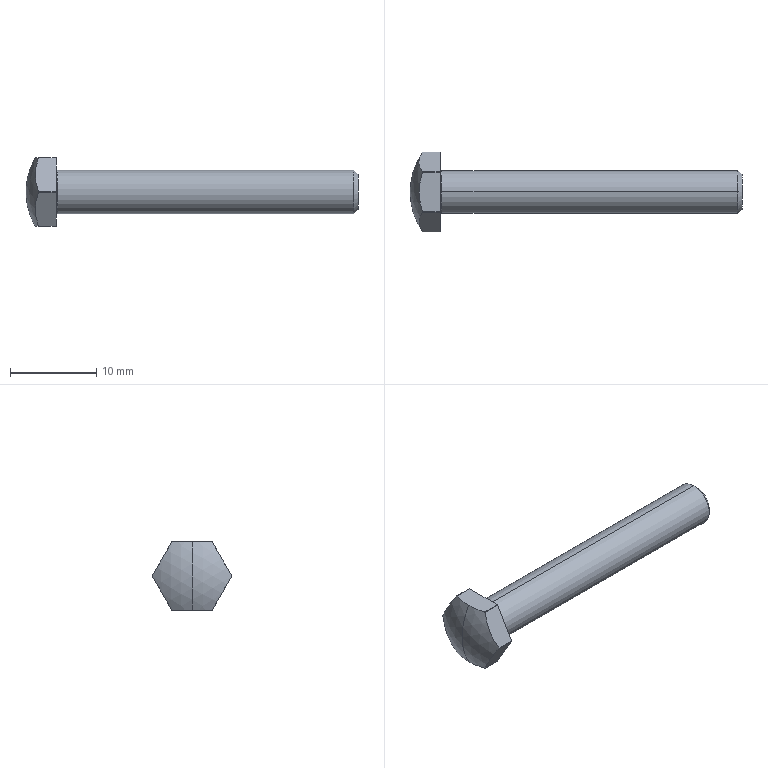Part | STEP file | 11-F12906-LQ-STBB5_35bA11 | 1 solid | 22 faces | box 38.5 x 9.2 x 8 mm | volume 847.17 mm3 | cylinder 8 | plane 8 | cone 2 | torus 2 | sphere 2 | commonest cylinder face diameters 9.2 x6 5 x2
STEP:
#1=CARTESIAN_POINT('',(35.,0.,2.01));
#2=VERTEX_POINT('',#1);
#3=CARTESIAN_POINT('',(35.,0.,-2.01));
#4=VERTEX_POINT('',#3);
#5=CARTESIAN_POINT('',(35.,0.,0.));
#6=DIRECTION('',(-1.,0.,0.));
#7=DIRECTION('',(0.,0.,1.));
#8=AXIS2_PLACEMENT_3D('',#5,#6,#7);
#9=CIRCLE('',#8,2.01);
#10=EDGE_CURVE('',#2,#4,#9,.T.);
#11=ORIENTED_EDGE('',*,*,#10,.T.);
#12=CARTESIAN_POINT('',(34.51,0.,-2.5));
#13=VERTEX_POINT('',#12);
#14=CARTESIAN_POINT('',(35.,0.,-2.01));
#15=DIRECTION('',(-0.7071,0.,-0.7071));
#16=VECTOR('',#15,1000.);
#17=LINE('',#14,#16);
#18=EDGE_CURVE('',#4,#13,#17,.T.);
#19=ORIENTED_EDGE('',*,*,#18,.T.);
#20=CARTESIAN_POINT('',(34.51,0.,2.5));
#21=VERTEX_POINT('',#20);
#22=CARTESIAN_POINT('',(34.51,0.,0.));
#23=DIRECTION('',(-1.,0.,0.));
#24=DIRECTION('',(0.,0.,1.));
#25=AXIS2_PLACEMENT_3D('',#22,#23,#24);
#26=CIRCLE('',#25,2.5);
#27=EDGE_CURVE('',#21,#13,#26,.T.);
#28=ORIENTED_EDGE('',*,*,#27,.F.);
#29=CARTESIAN_POINT('',(35.,0.,2.01));
#30=DIRECTION('',(-0.7071,0.,0.7071));
#31=VECTOR('',#30,1000.);
#32=LINE('',#29,#31);
#33=EDGE_CURVE('',#2,#21,#32,.T.);
#34=ORIENTED_EDGE('',*,*,#33,.F.);
#35=EDGE_LOOP('',(#11,#19,#28,#34));
#36=FACE_OUTER_BOUND('',#35,.T.);
#37=CARTESIAN_POINT('',(35.,0.,0.));
#38=DIRECTION('',(-1.,0.,0.));
#39=DIRECTION('',(0.,0.,1.));
#40=AXIS2_PLACEMENT_3D('',#37,#38,#39);
#41=CONICAL_SURFACE('',#40,2.01,0.7854);
#42=ADVANCED_FACE('',(#36),#41,.T.);
#43=ORIENTED_EDGE('',*,*,#27,.T.);
#44=CARTESIAN_POINT('',(0.2,0.,-2.5));
#45=VERTEX_POINT('',#44);
#46=CARTESIAN_POINT('',(35.,0.,-2.5));
#47=DIRECTION('',(-1.,0.,0.));
#48=VECTOR('',#47,1000.);
#49=LINE('',#46,#48);
#50=EDGE_CURVE('',#13,#45,#49,.T.);
#51=ORIENTED_EDGE('',*,*,#50,.T.);
#52=CARTESIAN_POINT('',(0.2,0.,2.5));
#53=VERTEX_POINT('',#52);
#54=CARTESIAN_POINT('',(0.2,0.,0.));
#55=DIRECTION('',(-1.,0.,0.));
#56=DIRECTION('',(0.,0.,1.));
#57=AXIS2_PLACEMENT_3D('',#54,#55,#56);
#58=CIRCLE('',#57,2.5);
#59=EDGE_CURVE('',#53,#45,#58,.T.);
#60=ORIENTED_EDGE('',*,*,#59,.F.);
#61=CARTESIAN_POINT('',(35.,0.,2.5));
#62=DIRECTION('',(-1.,0.,0.));
#63=VECTOR('',#62,1000.);
#64=LINE('',#61,#63);
#65=EDGE_CURVE('',#21,#53,#64,.T.);
#66=ORIENTED_EDGE('',*,*,#65,.F.);
#67=EDGE_LOOP('',(#43,#51,#60,#66));
#68=FACE_OUTER_BOUND('',#67,.T.);
#69=CARTESIAN_POINT('',(35.,0.,0.));
#70=DIRECTION('',(-1.,0.,0.));
#71=DIRECTION('',(0.,0.,1.));
#72=AXIS2_PLACEMENT_3D('',#69,#70,#71);
#73=CYLINDRICAL_SURFACE('',#72,2.5);
#74=ADVANCED_FACE('',(#68),#73,.T.);
#75=CARTESIAN_POINT('',(0.,0.,-2.7));
#76=VERTEX_POINT('',#75);
#77=CARTESIAN_POINT('',(0.,0.,2.7));
#78=VERTEX_POINT('',#77);
#79=CARTESIAN_POINT('',(0.,0.,0.));
#80=DIRECTION('',(-1.,0.,0.));
#81=DIRECTION('',(0.,0.,1.));
#82=AXIS2_PLACEMENT_3D('',#79,#80,#81);
#83=CIRCLE('',#82,2.7);
#84=EDGE_CURVE('',#76,#78,#83,.T.);
#85=ORIENTED_EDGE('',*,*,#84,.F.);
#86=CARTESIAN_POINT('',(0.2,0.,-2.7));
#87=DIRECTION('',(0.,1.,0.));
#88=DIRECTION('',(0.,0.,1.));
#89=AXIS2_PLACEMENT_3D('',#86,#87,#88);
#90=CIRCLE('',#89,0.2);
#91=EDGE_CURVE('',#76,#45,#90,.T.);
#92=ORIENTED_EDGE('',*,*,#91,.T.);
#93=CARTESIAN_POINT('',(0.2,0.,0.));
#94=DIRECTION('',(-1.,0.,0.));
#95=DIRECTION('',(0.,0.,1.));
#96=AXIS2_PLACEMENT_3D('',#93,#94,#95);
#97=CIRCLE('',#96,2.5);
#98=EDGE_CURVE('',#45,#53,#97,.T.);
#99=ORIENTED_EDGE('',*,*,#98,.T.);
#100=CARTESIAN_POINT('',(0.2,0.,2.7));
#101=DIRECTION('',(0.,-1.,0.));
#102=DIRECTION('',(0.,0.,-1.));
#103=AXIS2_PLACEMENT_3D('',#100,#101,#102);
#104=CIRCLE('',#103,0.2);
#105=EDGE_CURVE('',#78,#53,#104,.T.);
#106=ORIENTED_EDGE('',*,*,#105,.F.);
#107=EDGE_LOOP('',(#85,#92,#99,#106));
#108=FACE_OUTER_BOUND('',#107,.T.);
#109=CARTESIAN_POINT('',(0.2,0.,0.));
#110=DIRECTION('',(-1.,0.,0.));
#111=DIRECTION('',(0.,0.,1.));
#112=AXIS2_PLACEMENT_3D('',#109,#110,#111);
#113=TOROIDAL_SURFACE('',#112,2.7,0.2);
#114=ADVANCED_FACE('',(#108),#113,.F.);
#115=CARTESIAN_POINT('',(-2.428,0.,4.));
#116=VERTEX_POINT('',#115);
#117=CARTESIAN_POINT('',(-2.045,-2.272,4.));
#118=VERTEX_POINT('',#117);
#119=CARTESIAN_POINT('',(4.5,0.,4.));
#120=DIRECTION('',(0.,0.,1.));
#121=DIRECTION('',(1.,0.,0.));
#122=AXIS2_PLACEMENT_3D('',#119,#120,#121);
#123=CIRCLE('',#122,6.928);
#124=EDGE_CURVE('',#116,#118,#123,.T.);
#125=ORIENTED_EDGE('',*,*,#124,.F.);
#126=CARTESIAN_POINT('',(-3.5,0.,0.));
#127=VERTEX_POINT('',#126);
#128=CARTESIAN_POINT('',(4.5,0.,0.));
#129=DIRECTION('',(0.,-1.,0.));
#130=DIRECTION('',(0.,0.,-1.));
#131=AXIS2_PLACEMENT_3D('',#128,#129,#130);
#132=CIRCLE('',#131,8.);
#133=EDGE_CURVE('',#116,#127,#132,.T.);
#134=ORIENTED_EDGE('',*,*,#133,.T.);
#135=CARTESIAN_POINT('',(-2.428,0.,-4.));
#136=VERTEX_POINT('',#135);
#137=CARTESIAN_POINT('',(4.5,0.,0.));
#138=DIRECTION('',(0.,1.,0.));
#139=DIRECTION('',(0.,0.,1.));
#140=AXIS2_PLACEMENT_3D('',#137,#138,#139);
#141=CIRCLE('',#140,8.);
#142=EDGE_CURVE('',#136,#127,#141,.T.);
#143=ORIENTED_EDGE('',*,*,#142,.F.);
#144=CARTESIAN_POINT('',(-2.045,-2.272,-4.));
#145=VERTEX_POINT('',#144);
#146=CARTESIAN_POINT('',(4.5,0.,-4.));
#147=DIRECTION('',(0.,0.,-1.));
#148=DIRECTION('',(-1.,0.,0.));
#149=AXIS2_PLACEMENT_3D('',#146,#147,#148);
#150=CIRCLE('',#149,6.928);
#151=EDGE_CURVE('',#145,#136,#150,.T.);
#152=ORIENTED_EDGE('',*,*,#151,.F.);
#153=CARTESIAN_POINT('',(-2.045,-2.328,-3.967));
#154=VERTEX_POINT('',#153);
#155=CARTESIAN_POINT('',(-2.045,0.,0.));
#156=DIRECTION('',(-1.,0.,0.));
#157=DIRECTION('',(0.,0.,1.));
#158=AXIS2_PLACEMENT_3D('',#155,#156,#157);
#159=CIRCLE('',#158,4.6);
#160=EDGE_CURVE('',#145,#154,#159,.T.);
#161=ORIENTED_EDGE('',*,*,#160,.T.);
#162=CARTESIAN_POINT('',(-2.045,-4.6,-0.03277));
#163=VERTEX_POINT('',#162);
#164=CARTESIAN_POINT('',(4.5,-3.464,-2.));
#165=DIRECTION('',(0.,-0.866,-0.5));
#166=DIRECTION('',(0.,0.5,-0.866));
#167=AXIS2_PLACEMENT_3D('',#164,#165,#166);
#168=CIRCLE('',#167,6.928);
#169=EDGE_CURVE('',#163,#154,#168,.T.);
#170=ORIENTED_EDGE('',*,*,#169,.F.);
#171=CARTESIAN_POINT('',(-2.045,-4.6,0.03277));
#172=VERTEX_POINT('',#171);
#173=CARTESIAN_POINT('',(-2.045,0.,0.));
#174=DIRECTION('',(-1.,0.,0.));
#175=DIRECTION('',(0.,0.,1.));
#176=AXIS2_PLACEMENT_3D('',#173,#174,#175);
#177=CIRCLE('',#176,4.6);
#178=EDGE_CURVE('',#163,#172,#177,.T.);
#179=ORIENTED_EDGE('',*,*,#178,.T.);
#180=CARTESIAN_POINT('',(-2.045,-2.328,3.967));
#181=VERTEX_POINT('',#180);
#182=CARTESIAN_POINT('',(4.5,-3.464,2.));
#183=DIRECTION('',(0.,-0.866,0.5));
#184=DIRECTION('',(0.,-0.5,-0.866));
#185=AXIS2_PLACEMENT_3D('',#182,#183,#184);
#186=CIRCLE('',#185,6.928);
#187=EDGE_CURVE('',#181,#172,#186,.T.);
#188=ORIENTED_EDGE('',*,*,#187,.F.);
#189=CARTESIAN_POINT('',(-2.045,0.,0.));
#190=DIRECTION('',(-1.,0.,0.));
#191=DIRECTION('',(0.,0.,1.));
#192=AXIS2_PLACEMENT_3D('',#189,#190,#191);
#193=CIRCLE('',#192,4.6);
#194=EDGE_CURVE('',#181,#118,#193,.T.);
#195=ORIENTED_EDGE('',*,*,#194,.T.);
#196=EDGE_LOOP('',(#125,#134,#143,#152,#161,#170,#179,#188,#195));
#197=FACE_OUTER_BOUND('',#196,.T.);
#198=CARTESIAN_POINT('',(4.5,0.,0.));
#199=DIRECTION('',(0.,-1.,0.));
#200=DIRECTION('',(0.,0.,-1.));
#201=AXIS2_PLACEMENT_3D('',#198,#199,#200);
#202=SPHERICAL_SURFACE('',#201,8.);
#203=ADVANCED_FACE('',(#197),#202,.T.);
#204=ORIENTED_EDGE('',*,*,#133,.F.);
#205=CARTESIAN_POINT('',(-2.045,2.272,4.));
#206=VERTEX_POINT('',#205);
#207=CARTESIAN_POINT('',(4.5,0.,4.));
#208=DIRECTION('',(0.,0.,1.));
#209=DIRECTION('',(1.,0.,0.));
#210=AXIS2_PLACEMENT_3D('',#207,#208,#209);
#211=CIRCLE('',#210,6.928);
#212=EDGE_CURVE('',#206,#116,#211,.T.);
#213=ORIENTED_EDGE('',*,*,#212,.F.);
#214=CARTESIAN_POINT('',(-2.045,2.328,3.967));
#215=VERTEX_POINT('',#214);
#216=CARTESIAN_POINT('',(-2.045,0.,0.));
#217=DIRECTION('',(-1.,0.,0.));
#218=DIRECTION('',(0.,0.,1.));
#219=AXIS2_PLACEMENT_3D('',#216,#217,#218);
#220=CIRCLE('',#219,4.6);
#221=EDGE_CURVE('',#206,#215,#220,.T.);
#222=ORIENTED_EDGE('',*,*,#221,.T.);
#223=CARTESIAN_POINT('',(-2.045,4.6,0.03277));
#224=VERTEX_POINT('',#223);
#225=CARTESIAN_POINT('',(4.5,3.464,2.));
#226=DIRECTION('',(0.,0.866,0.5));
#227=DIRECTION('',(0.,-0.5,0.866));
#228=AXIS2_PLACEMENT_3D('',#225,#226,#227);
#229=CIRCLE('',#228,6.928);
#230=EDGE_CURVE('',#224,#215,#229,.T.);
#231=ORIENTED_EDGE('',*,*,#230,.F.);
#232=CARTESIAN_POINT('',(-2.045,4.6,-0.03277));
#233=VERTEX_POINT('',#232);
#234=CARTESIAN_POINT('',(-2.045,0.,0.));
#235=DIRECTION('',(-1.,0.,0.));
#236=DIRECTION('',(0.,0.,1.));
#237=AXIS2_PLACEMENT_3D('',#234,#235,#236);
#238=CIRCLE('',#237,4.6);
#239=EDGE_CURVE('',#224,#233,#238,.T.);
#240=ORIENTED_EDGE('',*,*,#239,.T.);
#241=CARTESIAN_POINT('',(-2.045,2.328,-3.967));
#242=VERTEX_POINT('',#241);
#243=CARTESIAN_POINT('',(4.5,3.464,-2.));
#244=DIRECTION('',(0.,0.866,-0.5));
#245=DIRECTION('',(0.,0.5,0.866));
#246=AXIS2_PLACEMENT_3D('',#243,#244,#245);
#247=CIRCLE('',#246,6.928);
#248=EDGE_CURVE('',#242,#233,#247,.T.);
#249=ORIENTED_EDGE('',*,*,#248,.F.);
#250=CARTESIAN_POINT('',(-2.045,2.272,-4.));
#251=VERTEX_POINT('',#250);
#252=CARTESIAN_POINT('',(-2.045,0.,0.));
#253=DIRECTION('',(-1.,0.,0.));
#254=DIRECTION('',(0.,0.,1.));
#255=AXIS2_PLACEMENT_3D('',#252,#253,#254);
#256=CIRCLE('',#255,4.6);
#257=EDGE_CURVE('',#242,#251,#256,.T.);
#258=ORIENTED_EDGE('',*,*,#257,.T.);
#259=CARTESIAN_POINT('',(4.5,0.,-4.));
#260=DIRECTION('',(0.,0.,-1.));
#261=DIRECTION('',(-1.,0.,0.));
#262=AXIS2_PLACEMENT_3D('',#259,#260,#261);
#263=CIRCLE('',#262,6.928);
#264=EDGE_CURVE('',#136,#251,#263,.T.);
#265=ORIENTED_EDGE('',*,*,#264,.F.);
#266=ORIENTED_EDGE('',*,*,#142,.T.);
#267=EDGE_LOOP('',(#204,#213,#222,#231,#240,#249,#258,#265,#266));
#268=FACE_OUTER_BOUND('',#267,.T.);
#269=CARTESIAN_POINT('',(4.5,0.,0.));
#270=DIRECTION('',(0.,-1.,0.));
#271=DIRECTION('',(0.,0.,-1.));
#272=AXIS2_PLACEMENT_3D('',#269,#270,#271);
#273=SPHERICAL_SURFACE('',#272,8.);
#274=ADVANCED_FACE('',(#268),#273,.T.);
#275=CARTESIAN_POINT('',(0.,4.6,0.03277));
#276=VERTEX_POINT('',#275);
#277=CARTESIAN_POINT('',(35.,4.6,0.03277));
#278=DIRECTION('',(-1.,0.,0.));
#279=VECTOR('',#278,1000.);
#280=LINE('',#277,#279);
#281=EDGE_CURVE('',#276,#224,#280,.T.);
#282=ORIENTED_EDGE('',*,*,#281,.F.);
#283=CARTESIAN_POINT('',(0.,4.6,-0.03277));
#284=VERTEX_POINT('',#283);
#285=CARTESIAN_POINT('',(0.,0.,0.));
#286=DIRECTION('',(-1.,0.,0.));
#287=DIRECTION('',(0.,0.,1.));
#288=AXIS2_PLACEMENT_3D('',#285,#286,#287);
#289=CIRCLE('',#288,4.6);
#290=EDGE_CURVE('',#276,#284,#289,.T.);
#291=ORIENTED_EDGE('',*,*,#290,.T.);
#292=CARTESIAN_POINT('',(35.,4.6,-0.03277));
#293=DIRECTION('',(1.,0.,0.));
#294=VECTOR('',#293,1000.);
#295=LINE('',#292,#294);
#296=EDGE_CURVE('',#233,#284,#295,.T.);
#297=ORIENTED_EDGE('',*,*,#296,.F.);
#298=ORIENTED_EDGE('',*,*,#239,.F.);
#299=EDGE_LOOP('',(#282,#291,#297,#298));
#300=FACE_OUTER_BOUND('',#299,.T.);
#301=CARTESIAN_POINT('',(35.,0.,0.));
#302=DIRECTION('',(-1.,0.,0.));
#303=DIRECTION('',(0.,0.,1.));
#304=AXIS2_PLACEMENT_3D('',#301,#302,#303);
#305=CYLINDRICAL_SURFACE('',#304,4.6);
#306=ADVANCED_FACE('',(#300),#305,.T.);
#307=CARTESIAN_POINT('',(0.,2.328,3.967));
#308=VERTEX_POINT('',#307);
#309=CARTESIAN_POINT('',(35.,2.328,3.967));
#310=DIRECTION('',(1.,0.,0.));
#311=VECTOR('',#310,1000.);
#312=LINE('',#309,#311);
#313=EDGE_CURVE('',#215,#308,#312,.T.);
#314=ORIENTED_EDGE('',*,*,#313,.F.);
#315=ORIENTED_EDGE('',*,*,#221,.F.);
#316=CARTESIAN_POINT('',(0.,2.272,4.));
#317=VERTEX_POINT('',#316);
#318=CARTESIAN_POINT('',(35.,2.272,4.));
#319=DIRECTION('',(-1.,0.,0.));
#320=VECTOR('',#319,1000.);
#321=LINE('',#318,#320);
#322=EDGE_CURVE('',#317,#206,#321,.T.);
#323=ORIENTED_EDGE('',*,*,#322,.F.);
#324=CARTESIAN_POINT('',(0.,0.,0.));
#325=DIRECTION('',(-1.,0.,0.));
#326=DIRECTION('',(0.,0.,1.));
#327=AXIS2_PLACEMENT_3D('',#324,#325,#326);
#328=CIRCLE('',#327,4.6);
#329=EDGE_CURVE('',#317,#308,#328,.T.);
#330=ORIENTED_EDGE('',*,*,#329,.T.);
#331=EDGE_LOOP('',(#314,#315,#323,#330));
#332=FACE_OUTER_BOUND('',#331,.T.);
#333=CARTESIAN_POINT('',(35.,0.,0.));
#334=DIRECTION('',(-1.,0.,0.));
#335=DIRECTION('',(0.,0.,1.));
#336=AXIS2_PLACEMENT_3D('',#333,#334,#335);
#337=CYLINDRICAL_SURFACE('',#336,4.6);
#338=ADVANCED_FACE('',(#332),#337,.T.);
#339=CARTESIAN_POINT('',(0.,2.328,-3.967));
#340=VERTEX_POINT('',#339);
#341=CARTESIAN_POINT('',(35.,2.328,-3.967));
#342=DIRECTION('',(-1.,0.,0.));
#343=VECTOR('',#342,1000.);
#344=LINE('',#341,#343);
#345=EDGE_CURVE('',#340,#242,#344,.T.);
#346=ORIENTED_EDGE('',*,*,#345,.F.);
#347=CARTESIAN_POINT('',(0.,2.272,-4.));
#348=VERTEX_POINT('',#347);
#349=CARTESIAN_POINT('',(0.,0.,0.));
#350=DIRECTION('',(-1.,0.,0.));
#351=DIRECTION('',(0.,0.,1.));
#352=AXIS2_PLACEMENT_3D('',#349,#350,#351);
#353=CIRCLE('',#352,4.6);
#354=EDGE_CURVE('',#340,#348,#353,.T.);
#355=ORIENTED_EDGE('',*,*,#354,.T.);
#356=CARTESIAN_POINT('',(35.,2.272,-4.));
#357=DIRECTION('',(1.,0.,0.));
#358=VECTOR('',#357,1000.);
#359=LINE('',#356,#358);
#360=EDGE_CURVE('',#251,#348,#359,.T.);
#361=ORIENTED_EDGE('',*,*,#360,.F.);
#362=ORIENTED_EDGE('',*,*,#257,.F.);
#363=EDGE_LOOP('',(#346,#355,#361,#362));
#364=FACE_OUTER_BOUND('',#363,.T.);
#365=CARTESIAN_POINT('',(35.,0.,0.));
#366=DIRECTION('',(-1.,0.,0.));
#367=DIRECTION('',(0.,0.,1.));
#368=AXIS2_PLACEMENT_3D('',#365,#366,#367);
#369=CYLINDRICAL_SURFACE('',#368,4.6);
#370=ADVANCED_FACE('',(#364),#369,.T.);
#371=CARTESIAN_POINT('',(0.,-2.272,-4.));
#372=VERTEX_POINT('',#371);
#373=CARTESIAN_POINT('',(35.,-2.272,-4.));
#374=DIRECTION('',(-1.,0.,0.));
#375=VECTOR('',#374,1000.);
#376=LINE('',#373,#375);
#377=EDGE_CURVE('',#372,#145,#376,.T.);
#378=ORIENTED_EDGE('',*,*,#377,.F.);
#379=CARTESIAN_POINT('',(0.,-2.328,-3.967));
#380=VERTEX_POINT('',#379);
#381=CARTESIAN_POINT('',(0.,0.,0.));
#382=DIRECTION('',(-1.,0.,0.));
#383=DIRECTION('',(0.,0.,1.));
#384=AXIS2_PLACEMENT_3D('',#381,#382,#383);
#385=CIRCLE('',#384,4.6);
#386=EDGE_CURVE('',#372,#380,#385,.T.);
#387=ORIENTED_EDGE('',*,*,#386,.T.);
#388=CARTESIAN_POINT('',(35.,-2.328,-3.967));
#389=DIRECTION('',(1.,0.,0.));
#390=VECTOR('',#389,1000.);
#391=LINE('',#388,#390);
#392=EDGE_CURVE('',#154,#380,#391,.T.);
#393=ORIENTED_EDGE('',*,*,#392,.F.);
#394=ORIENTED_EDGE('',*,*,#160,.F.);
#395=EDGE_LOOP('',(#378,#387,#393,#394));
#396=FACE_OUTER_BOUND('',#395,.T.);
#397=CARTESIAN_POINT('',(35.,0.,0.));
#398=DIRECTION('',(-1.,0.,0.));
#399=DIRECTION('',(0.,0.,1.));
#400=AXIS2_PLACEMENT_3D('',#397,#398,#399);
#401=CYLINDRICAL_SURFACE('',#400,4.6);
#402=ADVANCED_FACE('',(#396),#401,.T.);
#403=CARTESIAN_POINT('',(0.,-4.6,-0.03277));
#404=VERTEX_POINT('',#403);
#405=CARTESIAN_POINT('',(35.,-4.6,-0.03277));
#406=DIRECTION('',(-1.,0.,0.));
#407=VECTOR('',#406,1000.);
#408=LINE('',#405,#407);
#409=EDGE_CURVE('',#404,#163,#408,.T.);
#410=ORIENTED_EDGE('',*,*,#409,.F.);
#411=CARTESIAN_POINT('',(0.,-4.6,0.03277));
#412=VERTEX_POINT('',#411);
#413=CARTESIAN_POINT('',(0.,0.,0.));
#414=DIRECTION('',(-1.,0.,0.));
#415=DIRECTION('',(0.,0.,1.));
#416=AXIS2_PLACEMENT_3D('',#413,#414,#415);
#417=CIRCLE('',#416,4.6);
#418=EDGE_CURVE('',#404,#412,#417,.T.);
#419=ORIENTED_EDGE('',*,*,#418,.T.);
#420=CARTESIAN_POINT('',(35.,-4.6,0.03277));
#421=DIRECTION('',(1.,0.,0.));
#422=VECTOR('',#421,1000.);
#423=LINE('',#420,#422);
#424=EDGE_CURVE('',#172,#412,#423,.T.);
#425=ORIENTED_EDGE('',*,*,#424,.F.);
#426=ORIENTED_EDGE('',*,*,#178,.F.);
#427=EDGE_LOOP('',(#410,#419,#425,#426));
#428=FACE_OUTER_BOUND('',#427,.T.);
#429=CARTESIAN_POINT('',(35.,0.,0.));
#430=DIRECTION('',(-1.,0.,0.));
#431=DIRECTION('',(0.,0.,1.));
#432=AXIS2_PLACEMENT_3D('',#429,#430,#431);
#433=CYLINDRICAL_SURFACE('',#432,4.6);
#434=ADVANCED_FACE('',(#428),#433,.T.);
#435=CARTESIAN_POINT('',(0.,-2.328,3.967));
#436=VERTEX_POINT('',#435);
#437=CARTESIAN_POINT('',(35.,-2.328,3.967));
#438=DIRECTION('',(-1.,0.,0.));
#439=VECTOR('',#438,1000.);
#440=LINE('',#437,#439);
#441=EDGE_CURVE('',#436,#181,#440,.T.);
#442=ORIENTED_EDGE('',*,*,#441,.F.);
#443=CARTESIAN_POINT('',(0.,-2.272,4.));
#444=VERTEX_POINT('',#443);
#445=CARTESIAN_POINT('',(0.,0.,0.));
#446=DIRECTION('',(-1.,0.,0.));
#447=DIRECTION('',(0.,0.,1.));
#448=AXIS2_PLACEMENT_3D('',#445,#446,#447);
#449=CIRCLE('',#448,4.6);
#450=EDGE_CURVE('',#436,#444,#449,.T.);
#451=ORIENTED_EDGE('',*,*,#450,.T.);
#452=CARTESIAN_POINT('',(35.,-2.272,4.));
#453=DIRECTION('',(1.,0.,0.));
#454=VECTOR('',#453,1000.);
#455=LINE('',#452,#454);
#456=EDGE_CURVE('',#118,#444,#455,.T.);
#457=ORIENTED_EDGE('',*,*,#456,.F.);
#458=ORIENTED_EDGE('',*,*,#194,.F.);
#459=EDGE_LOOP('',(#442,#451,#457,#458));
#460=FACE_OUTER_BOUND('',#459,.T.);
#461=CARTESIAN_POINT('',(35.,0.,0.));
#462=DIRECTION('',(-1.,0.,0.));
#463=DIRECTION('',(0.,0.,1.));
#464=AXIS2_PLACEMENT_3D('',#461,#462,#463);
#465=CYLINDRICAL_SURFACE('',#464,4.6);
#466=ADVANCED_FACE('',(#460),#465,.T.);
#467=CARTESIAN_POINT('',(0.,0.,0.));
#468=DIRECTION('',(-1.,0.,0.));
#469=DIRECTION('',(0.,0.,1.));
#470=AXIS2_PLACEMENT_3D('',#467,#468,#469);
#471=CIRCLE('',#470,2.7);
#472=EDGE_CURVE('',#78,#76,#471,.T.);
#473=ORIENTED_EDGE('',*,*,#472,.T.);
#474=ORIENTED_EDGE('',*,*,#84,.T.);
#475=EDGE_LOOP('',(#473,#474));
#476=FACE_BOUND('',#475,.T.);
#477=CARTESIAN_POINT('',(0.,5.456,-1.45));
#478=DIRECTION('',(0.,0.5,-0.866));
#479=VECTOR('',#478,1000.);
#480=LINE('',#477,#479);
#481=EDGE_CURVE('',#308,#276,#480,.T.);
#482=ORIENTED_EDGE('',*,*,#481,.F.);
#483=ORIENTED_EDGE('',*,*,#329,.F.);
#484=CARTESIAN_POINT('',(0.,0.,4.));
#485=DIRECTION('',(0.,1.,0.));
#486=VECTOR('',#485,1000.);
#487=LINE('',#484,#486);
#488=EDGE_CURVE('',#444,#317,#487,.T.);
#489=ORIENTED_EDGE('',*,*,#488,.F.);
#490=ORIENTED_EDGE('',*,*,#450,.F.);
#491=CARTESIAN_POINT('',(0.,-5.456,-1.45));
#492=DIRECTION('',(0.,0.5,0.866));
#493=VECTOR('',#492,1000.);
#494=LINE('',#491,#493);
#495=EDGE_CURVE('',#412,#436,#494,.T.);
#496=ORIENTED_EDGE('',*,*,#495,.F.);
#497=ORIENTED_EDGE('',*,*,#418,.F.);
#498=CARTESIAN_POINT('',(0.,-1.472,-5.45));
#499=DIRECTION('',(0.,-0.5,0.866));
#500=VECTOR('',#499,1000.);
#501=LINE('',#498,#500);
#502=EDGE_CURVE('',#380,#404,#501,.T.);
#503=ORIENTED_EDGE('',*,*,#502,.F.);
#504=ORIENTED_EDGE('',*,*,#386,.F.);
#505=CARTESIAN_POINT('',(0.,0.,-4.));
#506=DIRECTION('',(0.,-1.,0.));
#507=VECTOR('',#506,1000.);
#508=LINE('',#505,#507);
#509=EDGE_CURVE('',#348,#372,#508,.T.);
#510=ORIENTED_EDGE('',*,*,#509,.F.);
#511=ORIENTED_EDGE('',*,*,#354,.F.);
#512=CARTESIAN_POINT('',(0.,1.472,-5.45));
#513=DIRECTION('',(0.,-0.5,-0.866));
#514=VECTOR('',#513,1000.);
#515=LINE('',#512,#514);
#516=EDGE_CURVE('',#284,#340,#515,.T.);
#517=ORIENTED_EDGE('',*,*,#516,.F.);
#518=ORIENTED_EDGE('',*,*,#290,.F.);
#519=EDGE_LOOP('',(#482,#483,#489,#490,#496,#497,#503,#504,#510,#511,#517,#518));
#520=FACE_OUTER_BOUND('',#519,.T.);
#521=CARTESIAN_POINT('',(0.,0.,-4.6));
#522=DIRECTION('',(-1.,0.,0.));
#523=DIRECTION('',(0.,0.,1.));
#524=AXIS2_PLACEMENT_3D('',#521,#522,#523);
#525=PLANE('',#524);
#526=ADVANCED_FACE('',(#476,#520),#525,.F.);
#527=ORIENTED_EDGE('',*,*,#91,.F.);
#528=ORIENTED_EDGE('',*,*,#472,.F.);
#529=ORIENTED_EDGE('',*,*,#105,.T.);
#530=ORIENTED_EDGE('',*,*,#59,.T.);
#531=EDGE_LOOP('',(#527,#528,#529,#530));
#532=FACE_OUTER_BOUND('',#531,.T.);
#533=CARTESIAN_POINT('',(0.2,0.,0.));
#534=DIRECTION('',(-1.,0.,0.));
#535=DIRECTION('',(0.,0.,1.));
#536=AXIS2_PLACEMENT_3D('',#533,#534,#535);
#537=TOROIDAL_SURFACE('',#536,2.7,0.2);
#538=ADVANCED_FACE('',(#532),#537,.F.);
#539=ORIENTED_EDGE('',*,*,#50,.F.);
#540=CARTESIAN_POINT('',(34.51,0.,0.));
#541=DIRECTION('',(-1.,0.,0.));
#542=DIRECTION('',(0.,0.,1.));
#543=AXIS2_PLACEMENT_3D('',#540,#541,#542);
#544=CIRCLE('',#543,2.5);
#545=EDGE_CURVE('',#13,#21,#544,.T.);
#546=ORIENTED_EDGE('',*,*,#545,.T.);
#547=ORIENTED_EDGE('',*,*,#65,.T.);
#548=ORIENTED_EDGE('',*,*,#98,.F.);
#549=EDGE_LOOP('',(#539,#546,#547,#548));
#550=FACE_OUTER_BOUND('',#549,.T.);
#551=CARTESIAN_POINT('',(35.,0.,0.));
#552=DIRECTION('',(-1.,0.,0.));
#553=DIRECTION('',(0.,0.,1.));
#554=AXIS2_PLACEMENT_3D('',#551,#552,#553);
#555=CYLINDRICAL_SURFACE('',#554,2.5);
#556=ADVANCED_FACE('',(#550),#555,.T.);
#557=ORIENTED_EDGE('',*,*,#18,.F.);
#558=CARTESIAN_POINT('',(35.,0.,0.));
#559=DIRECTION('',(-1.,0.,0.));
#560=DIRECTION('',(0.,0.,1.));
#561=AXIS2_PLACEMENT_3D('',#558,#559,#560);
#562=CIRCLE('',#561,2.01);
#563=EDGE_CURVE('',#4,#2,#562,.T.);
#564=ORIENTED_EDGE('',*,*,#563,.T.);
#565=ORIENTED_EDGE('',*,*,#33,.T.);
#566=ORIENTED_EDGE('',*,*,#545,.F.);
#567=EDGE_LOOP('',(#557,#564,#565,#566));
#568=FACE_OUTER_BOUND('',#567,.T.);
#569=CARTESIAN_POINT('',(35.,0.,0.));
#570=DIRECTION('',(-1.,0.,0.));
#571=DIRECTION('',(0.,0.,1.));
#572=AXIS2_PLACEMENT_3D('',#569,#570,#571);
#573=CONICAL_SURFACE('',#572,2.01,0.7854);
#574=ADVANCED_FACE('',(#568),#573,.T.);
#575=ORIENTED_EDGE('',*,*,#10,.F.);
#576=ORIENTED_EDGE('',*,*,#563,.F.);
#577=EDGE_LOOP('',(#575,#576));
#578=FACE_OUTER_BOUND('',#577,.T.);
#579=CARTESIAN_POINT('',(35.,0.,-2.01));
#580=DIRECTION('',(-1.,0.,0.));
#581=DIRECTION('',(0.,0.,1.));
#582=AXIS2_PLACEMENT_3D('',#579,#580,#581);
#583=PLANE('',#582);
#584=ADVANCED_FACE('',(#578),#583,.F.);
#585=ORIENTED_EDGE('',*,*,#322,.T.);
#586=ORIENTED_EDGE('',*,*,#212,.T.);
#587=ORIENTED_EDGE('',*,*,#124,.T.);
#588=ORIENTED_EDGE('',*,*,#456,.T.);
#589=ORIENTED_EDGE('',*,*,#488,.T.);
#590=EDGE_LOOP('',(#585,#586,#587,#588,#589));
#591=FACE_OUTER_BOUND('',#590,.T.);
#592=CARTESIAN_POINT('',(-3.5,2.309,4.));
#593=DIRECTION('',(0.,0.,1.));
#594=DIRECTION('',(1.,0.,0.));
#595=AXIS2_PLACEMENT_3D('',#592,#593,#594);
#596=PLANE('',#595);
#597=ADVANCED_FACE('',(#591),#596,.T.);
#598=ORIENTED_EDGE('',*,*,#441,.T.);
#599=ORIENTED_EDGE('',*,*,#187,.T.);
#600=ORIENTED_EDGE('',*,*,#424,.T.);
#601=ORIENTED_EDGE('',*,*,#495,.T.);
#602=EDGE_LOOP('',(#598,#599,#600,#601));
#603=FACE_OUTER_BOUND('',#602,.T.);
#604=CARTESIAN_POINT('',(-3.5,-2.309,4.));
#605=DIRECTION('',(0.,-0.866,0.5));
#606=DIRECTION('',(0.,-0.5,-0.866));
#607=AXIS2_PLACEMENT_3D('',#604,#605,#606);
#608=PLANE('',#607);
#609=ADVANCED_FACE('',(#603),#608,.T.);
#610=ORIENTED_EDGE('',*,*,#409,.T.);
#611=ORIENTED_EDGE('',*,*,#169,.T.);
#612=ORIENTED_EDGE('',*,*,#392,.T.);
#613=ORIENTED_EDGE('',*,*,#502,.T.);
#614=EDGE_LOOP('',(#610,#611,#612,#613));
#615=FACE_OUTER_BOUND('',#614,.T.);
#616=CARTESIAN_POINT('',(-3.5,-4.619,0.));
#617=DIRECTION('',(0.,-0.866,-0.5));
#618=DIRECTION('',(0.,0.5,-0.866));
#619=AXIS2_PLACEMENT_3D('',#616,#617,#618);
#620=PLANE('',#619);
#621=ADVANCED_FACE('',(#615),#620,.T.);
#622=ORIENTED_EDGE('',*,*,#377,.T.);
#623=ORIENTED_EDGE('',*,*,#151,.T.);
#624=ORIENTED_EDGE('',*,*,#264,.T.);
#625=ORIENTED_EDGE('',*,*,#360,.T.);
#626=ORIENTED_EDGE('',*,*,#509,.T.);
#627=EDGE_LOOP('',(#622,#623,#624,#625,#626));
#628=FACE_OUTER_BOUND('',#627,.T.);
#629=CARTESIAN_POINT('',(-3.5,-2.309,-4.));
#630=DIRECTION('',(0.,0.,-1.));
#631=DIRECTION('',(-1.,0.,0.));
#632=AXIS2_PLACEMENT_3D('',#629,#630,#631);
#633=PLANE('',#632);
#634=ADVANCED_FACE('',(#628),#633,.T.);
#635=ORIENTED_EDGE('',*,*,#345,.T.);
#636=ORIENTED_EDGE('',*,*,#248,.T.);
#637=ORIENTED_EDGE('',*,*,#296,.T.);
#638=ORIENTED_EDGE('',*,*,#516,.T.);
#639=EDGE_LOOP('',(#635,#636,#637,#638));
#640=FACE_OUTER_BOUND('',#639,.T.);
#641=CARTESIAN_POINT('',(-3.5,2.309,-4.));
#642=DIRECTION('',(0.,0.866,-0.5));
#643=DIRECTION('',(0.,0.5,0.866));
#644=AXIS2_PLACEMENT_3D('',#641,#642,#643);
#645=PLANE('',#644);
#646=ADVANCED_FACE('',(#640),#645,.T.);
#647=ORIENTED_EDGE('',*,*,#281,.T.);
#648=ORIENTED_EDGE('',*,*,#230,.T.);
#649=ORIENTED_EDGE('',*,*,#313,.T.);
#650=ORIENTED_EDGE('',*,*,#481,.T.);
#651=EDGE_LOOP('',(#647,#648,#649,#650));
#652=FACE_OUTER_BOUND('',#651,.T.);
#653=CARTESIAN_POINT('',(-3.5,4.619,0.));
#654=DIRECTION('',(0.,0.866,0.5));
#655=DIRECTION('',(0.,-0.5,0.866));
#656=AXIS2_PLACEMENT_3D('',#653,#654,#655);
#657=PLANE('',#656);
#658=ADVANCED_FACE('',(#652),#657,.T.);
#659=CLOSED_SHELL('',(#42,#74,#114,#203,#274,#306,#338,#370,#402,#434,#466,#526,#538,#556,#574,#584,#597,#609,#621,#634,#646,#658));
#660=MANIFOLD_SOLID_BREP('',#659);
#661=CARTESIAN_POINT('',(0.,0.,0.));
#662=DIRECTION('',(0.,0.,1.));
#663=DIRECTION('',(1.,0.,0.));
#664=AXIS2_PLACEMENT_3D('',#661,#662,#663);
#665=(LENGTH_UNIT()NAMED_UNIT(*)SI_UNIT(.MILLI.,.METRE.));
#666=UNCERTAINTY_MEASURE_WITH_UNIT(LENGTH_MEASURE(0.00001),#665,'','');
#667=(NAMED_UNIT(*)PLANE_ANGLE_UNIT()SI_UNIT($,.RADIAN.));
#668=(NAMED_UNIT(*)SI_UNIT($,.STERADIAN.)SOLID_ANGLE_UNIT());
#669=(GEOMETRIC_REPRESENTATION_CONTEXT(3)GLOBAL_UNCERTAINTY_ASSIGNED_CONTEXT((#666))GLOBAL_UNIT_ASSIGNED_CONTEXT((#665,#667,#668))REPRESENTATION_CONTEXT('',''));
#670=ADVANCED_BREP_SHAPE_REPRESENTATION('',(#660,#664),#669);